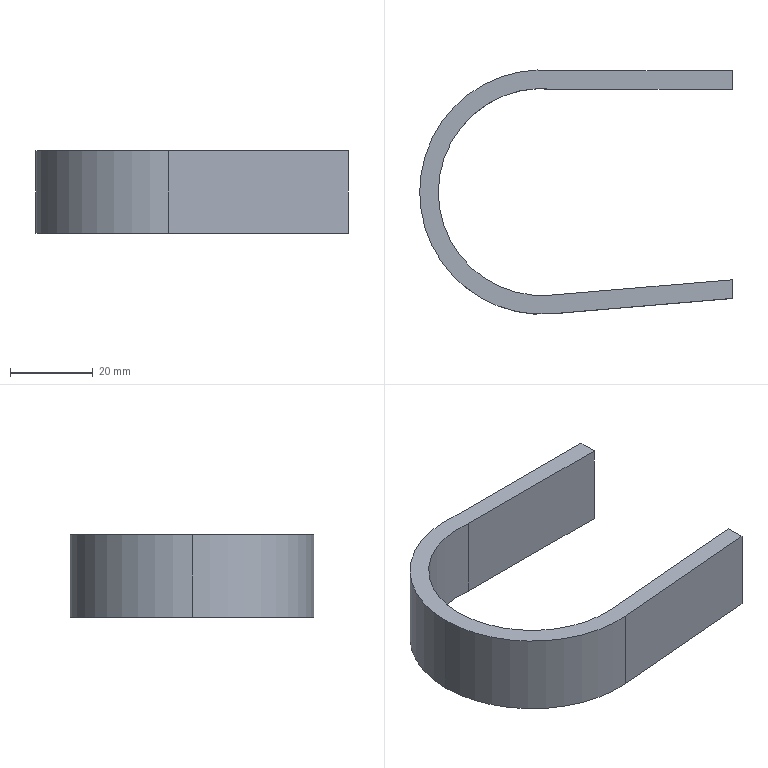Part | STEP file | Guide wheel mechanism revised.sldasm-Part-89 | 1 solid | 12 faces | box 75.5 x 59 x 20 mm | volume 15993 mm3 | plane 8 | cylinder 4 | commonest cylinder face diameters 50 x2 59 x2
STEP:
#1=CARTESIAN_POINT('',(-32.907,-0.3917,10.));
#2=VERTEX_POINT('',#1);
#3=CARTESIAN_POINT('',(-4.83,24.418,10.));
#4=VERTEX_POINT('',#3);
#5=CARTESIAN_POINT('',(-7.907,-0.3917,10.));
#6=DIRECTION('',(0.,0.,-1.));
#7=DIRECTION('',(1.,0.,0.));
#8=AXIS2_PLACEMENT_3D('',#5,#6,#7);
#9=CIRCLE('',#8,25.);
#10=EDGE_CURVE('',#2,#4,#9,.T.);
#11=ORIENTED_EDGE('',*,*,#10,.F.);
#12=CARTESIAN_POINT('',(-32.907,-0.3917,-10.));
#13=VERTEX_POINT('',#12);
#14=CARTESIAN_POINT('',(-32.907,-0.3917,10.));
#15=DIRECTION('',(0.,0.,-1.));
#16=VECTOR('',#15,1000.);
#17=LINE('',#14,#16);
#18=EDGE_CURVE('',#2,#13,#17,.T.);
#19=ORIENTED_EDGE('',*,*,#18,.T.);
#20=CARTESIAN_POINT('',(-4.83,24.418,-10.));
#21=VERTEX_POINT('',#20);
#22=CARTESIAN_POINT('',(-7.907,-0.3917,-10.));
#23=DIRECTION('',(0.,0.,-1.));
#24=DIRECTION('',(1.,0.,0.));
#25=AXIS2_PLACEMENT_3D('',#22,#23,#24);
#26=CIRCLE('',#25,25.);
#27=EDGE_CURVE('',#13,#21,#26,.T.);
#28=ORIENTED_EDGE('',*,*,#27,.T.);
#29=CARTESIAN_POINT('',(-4.83,24.418,10.));
#30=DIRECTION('',(0.,0.,-1.));
#31=VECTOR('',#30,1000.);
#32=LINE('',#29,#31);
#33=EDGE_CURVE('',#4,#21,#32,.T.);
#34=ORIENTED_EDGE('',*,*,#33,.F.);
#35=EDGE_LOOP('',(#11,#19,#28,#34));
#36=FACE_OUTER_BOUND('',#35,.T.);
#37=CARTESIAN_POINT('',(-7.907,-0.3917,10.));
#38=DIRECTION('',(0.,0.,-1.));
#39=DIRECTION('',(-1.,0.,0.));
#40=AXIS2_PLACEMENT_3D('',#37,#38,#39);
#41=CYLINDRICAL_SURFACE('',#40,25.);
#42=ADVANCED_FACE('',(#36),#41,.F.);
#43=CARTESIAN_POINT('',(-37.407,-0.3917,10.));
#44=VERTEX_POINT('',#43);
#45=CARTESIAN_POINT('',(-5.405,-29.785,10.));
#46=VERTEX_POINT('',#45);
#47=CARTESIAN_POINT('',(-7.907,-0.3917,10.));
#48=DIRECTION('',(0.,0.,1.));
#49=DIRECTION('',(1.,0.,0.));
#50=AXIS2_PLACEMENT_3D('',#47,#48,#49);
#51=CIRCLE('',#50,29.5);
#52=EDGE_CURVE('',#44,#46,#51,.T.);
#53=ORIENTED_EDGE('',*,*,#52,.F.);
#54=CARTESIAN_POINT('',(-37.407,-0.3917,-10.));
#55=VERTEX_POINT('',#54);
#56=CARTESIAN_POINT('',(-37.407,-0.3917,10.));
#57=DIRECTION('',(0.,0.,-1.));
#58=VECTOR('',#57,1000.);
#59=LINE('',#56,#58);
#60=EDGE_CURVE('',#44,#55,#59,.T.);
#61=ORIENTED_EDGE('',*,*,#60,.T.);
#62=CARTESIAN_POINT('',(-5.405,-29.785,-10.));
#63=VERTEX_POINT('',#62);
#64=CARTESIAN_POINT('',(-7.907,-0.3917,-10.));
#65=DIRECTION('',(0.,0.,1.));
#66=DIRECTION('',(1.,0.,0.));
#67=AXIS2_PLACEMENT_3D('',#64,#65,#66);
#68=CIRCLE('',#67,29.5);
#69=EDGE_CURVE('',#55,#63,#68,.T.);
#70=ORIENTED_EDGE('',*,*,#69,.T.);
#71=CARTESIAN_POINT('',(-5.405,-29.785,10.));
#72=DIRECTION('',(0.,0.,-1.));
#73=VECTOR('',#72,1000.);
#74=LINE('',#71,#73);
#75=EDGE_CURVE('',#46,#63,#74,.T.);
#76=ORIENTED_EDGE('',*,*,#75,.F.);
#77=EDGE_LOOP('',(#53,#61,#70,#76));
#78=FACE_OUTER_BOUND('',#77,.T.);
#79=CARTESIAN_POINT('',(-7.907,-0.3917,10.));
#80=DIRECTION('',(0.,0.,-1.));
#81=DIRECTION('',(-1.,0.,0.));
#82=AXIS2_PLACEMENT_3D('',#79,#80,#81);
#83=CYLINDRICAL_SURFACE('',#82,29.5);
#84=ADVANCED_FACE('',(#78),#83,.T.);
#85=CARTESIAN_POINT('',(38.093,24.418,-10.));
#86=VERTEX_POINT('',#85);
#87=CARTESIAN_POINT('',(38.093,28.918,-10.));
#88=VERTEX_POINT('',#87);
#89=CARTESIAN_POINT('',(38.093,28.918,-10.));
#90=DIRECTION('',(0.,1.,0.));
#91=VECTOR('',#90,1000.);
#92=LINE('',#89,#91);
#93=EDGE_CURVE('',#86,#88,#92,.T.);
#94=ORIENTED_EDGE('',*,*,#93,.T.);
#95=CARTESIAN_POINT('',(38.093,28.918,10.));
#96=VERTEX_POINT('',#95);
#97=CARTESIAN_POINT('',(38.093,28.918,10.));
#98=DIRECTION('',(0.,0.,-1.));
#99=VECTOR('',#98,1000.);
#100=LINE('',#97,#99);
#101=EDGE_CURVE('',#96,#88,#100,.T.);
#102=ORIENTED_EDGE('',*,*,#101,.F.);
#103=CARTESIAN_POINT('',(38.093,24.418,10.));
#104=VERTEX_POINT('',#103);
#105=CARTESIAN_POINT('',(38.093,28.918,10.));
#106=DIRECTION('',(0.,1.,0.));
#107=VECTOR('',#106,1000.);
#108=LINE('',#105,#107);
#109=EDGE_CURVE('',#104,#96,#108,.T.);
#110=ORIENTED_EDGE('',*,*,#109,.F.);
#111=CARTESIAN_POINT('',(38.093,24.418,10.));
#112=DIRECTION('',(0.,0.,-1.));
#113=VECTOR('',#112,1000.);
#114=LINE('',#111,#113);
#115=EDGE_CURVE('',#104,#86,#114,.T.);
#116=ORIENTED_EDGE('',*,*,#115,.T.);
#117=EDGE_LOOP('',(#94,#102,#110,#116));
#118=FACE_OUTER_BOUND('',#117,.T.);
#119=CARTESIAN_POINT('',(38.093,28.918,10.));
#120=DIRECTION('',(-1.,0.,0.));
#121=DIRECTION('',(0.,0.,1.));
#122=AXIS2_PLACEMENT_3D('',#119,#120,#121);
#123=PLANE('',#122);
#124=ADVANCED_FACE('',(#118),#123,.F.);
#125=CARTESIAN_POINT('',(-4.564,28.918,-10.));
#126=VERTEX_POINT('',#125);
#127=CARTESIAN_POINT('',(38.093,28.918,-10.));
#128=DIRECTION('',(-1.,0.,0.));
#129=VECTOR('',#128,1000.);
#130=LINE('',#127,#129);
#131=EDGE_CURVE('',#88,#126,#130,.T.);
#132=ORIENTED_EDGE('',*,*,#131,.T.);
#133=CARTESIAN_POINT('',(-4.564,28.918,10.));
#134=VERTEX_POINT('',#133);
#135=CARTESIAN_POINT('',(-4.564,28.918,10.));
#136=DIRECTION('',(0.,0.,-1.));
#137=VECTOR('',#136,1000.);
#138=LINE('',#135,#137);
#139=EDGE_CURVE('',#134,#126,#138,.T.);
#140=ORIENTED_EDGE('',*,*,#139,.F.);
#141=CARTESIAN_POINT('',(38.093,28.918,10.));
#142=DIRECTION('',(-1.,0.,0.));
#143=VECTOR('',#142,1000.);
#144=LINE('',#141,#143);
#145=EDGE_CURVE('',#96,#134,#144,.T.);
#146=ORIENTED_EDGE('',*,*,#145,.F.);
#147=ORIENTED_EDGE('',*,*,#101,.T.);
#148=EDGE_LOOP('',(#132,#140,#146,#147));
#149=FACE_OUTER_BOUND('',#148,.T.);
#150=CARTESIAN_POINT('',(38.093,28.918,10.));
#151=DIRECTION('',(0.,-1.,0.));
#152=DIRECTION('',(1.,0.,0.));
#153=AXIS2_PLACEMENT_3D('',#150,#151,#152);
#154=PLANE('',#153);
#155=ADVANCED_FACE('',(#149),#154,.F.);
#156=ORIENTED_EDGE('',*,*,#60,.F.);
#157=CARTESIAN_POINT('',(-7.907,-0.3917,10.));
#158=DIRECTION('',(0.,0.,1.));
#159=DIRECTION('',(1.,0.,0.));
#160=AXIS2_PLACEMENT_3D('',#157,#158,#159);
#161=CIRCLE('',#160,29.5);
#162=EDGE_CURVE('',#134,#44,#161,.T.);
#163=ORIENTED_EDGE('',*,*,#162,.F.);
#164=ORIENTED_EDGE('',*,*,#139,.T.);
#165=CARTESIAN_POINT('',(-7.907,-0.3917,-10.));
#166=DIRECTION('',(0.,0.,1.));
#167=DIRECTION('',(1.,0.,0.));
#168=AXIS2_PLACEMENT_3D('',#165,#166,#167);
#169=CIRCLE('',#168,29.5);
#170=EDGE_CURVE('',#126,#55,#169,.T.);
#171=ORIENTED_EDGE('',*,*,#170,.T.);
#172=EDGE_LOOP('',(#156,#163,#164,#171));
#173=FACE_OUTER_BOUND('',#172,.T.);
#174=CARTESIAN_POINT('',(-7.907,-0.3917,10.));
#175=DIRECTION('',(0.,0.,-1.));
#176=DIRECTION('',(-1.,0.,0.));
#177=AXIS2_PLACEMENT_3D('',#174,#175,#176);
#178=CYLINDRICAL_SURFACE('',#177,29.5);
#179=ADVANCED_FACE('',(#173),#178,.T.);
#180=CARTESIAN_POINT('',(38.093,-26.082,-10.));
#181=VERTEX_POINT('',#180);
#182=CARTESIAN_POINT('',(38.093,-26.082,-10.));
#183=DIRECTION('',(0.9964,0.08484,0.));
#184=VECTOR('',#183,1000.);
#185=LINE('',#182,#184);
#186=EDGE_CURVE('',#63,#181,#185,.T.);
#187=ORIENTED_EDGE('',*,*,#186,.T.);
#188=CARTESIAN_POINT('',(38.093,-26.082,10.));
#189=VERTEX_POINT('',#188);
#190=CARTESIAN_POINT('',(38.093,-26.082,10.));
#191=DIRECTION('',(0.,0.,-1.));
#192=VECTOR('',#191,1000.);
#193=LINE('',#190,#192);
#194=EDGE_CURVE('',#189,#181,#193,.T.);
#195=ORIENTED_EDGE('',*,*,#194,.F.);
#196=CARTESIAN_POINT('',(38.093,-26.082,10.));
#197=DIRECTION('',(0.9964,0.08484,0.));
#198=VECTOR('',#197,1000.);
#199=LINE('',#196,#198);
#200=EDGE_CURVE('',#46,#189,#199,.T.);
#201=ORIENTED_EDGE('',*,*,#200,.F.);
#202=ORIENTED_EDGE('',*,*,#75,.T.);
#203=EDGE_LOOP('',(#187,#195,#201,#202));
#204=FACE_OUTER_BOUND('',#203,.T.);
#205=CARTESIAN_POINT('',(38.093,-26.082,10.));
#206=DIRECTION('',(-0.08484,0.9964,0.));
#207=DIRECTION('',(-0.9964,-0.08484,0.));
#208=AXIS2_PLACEMENT_3D('',#205,#206,#207);
#209=PLANE('',#208);
#210=ADVANCED_FACE('',(#204),#209,.F.);
#211=CARTESIAN_POINT('',(38.093,-21.582,-10.));
#212=VERTEX_POINT('',#211);
#213=CARTESIAN_POINT('',(38.093,-21.582,-10.));
#214=DIRECTION('',(0.,1.,0.));
#215=VECTOR('',#214,1000.);
#216=LINE('',#213,#215);
#217=EDGE_CURVE('',#181,#212,#216,.T.);
#218=ORIENTED_EDGE('',*,*,#217,.T.);
#219=CARTESIAN_POINT('',(38.093,-21.582,10.));
#220=VERTEX_POINT('',#219);
#221=CARTESIAN_POINT('',(38.093,-21.582,10.));
#222=DIRECTION('',(0.,0.,-1.));
#223=VECTOR('',#222,1000.);
#224=LINE('',#221,#223);
#225=EDGE_CURVE('',#220,#212,#224,.T.);
#226=ORIENTED_EDGE('',*,*,#225,.F.);
#227=CARTESIAN_POINT('',(38.093,-21.582,10.));
#228=DIRECTION('',(0.,1.,0.));
#229=VECTOR('',#228,1000.);
#230=LINE('',#227,#229);
#231=EDGE_CURVE('',#189,#220,#230,.T.);
#232=ORIENTED_EDGE('',*,*,#231,.F.);
#233=ORIENTED_EDGE('',*,*,#194,.T.);
#234=EDGE_LOOP('',(#218,#226,#232,#233));
#235=FACE_OUTER_BOUND('',#234,.T.);
#236=CARTESIAN_POINT('',(38.093,-21.582,10.));
#237=DIRECTION('',(-1.,0.,0.));
#238=DIRECTION('',(0.,0.,1.));
#239=AXIS2_PLACEMENT_3D('',#236,#237,#238);
#240=PLANE('',#239);
#241=ADVANCED_FACE('',(#235),#240,.F.);
#242=CARTESIAN_POINT('',(-5.796,-25.302,-10.));
#243=VERTEX_POINT('',#242);
#244=CARTESIAN_POINT('',(38.093,-21.582,-10.));
#245=DIRECTION('',(-0.9964,-0.08447,0.));
#246=VECTOR('',#245,1000.);
#247=LINE('',#244,#246);
#248=EDGE_CURVE('',#212,#243,#247,.T.);
#249=ORIENTED_EDGE('',*,*,#248,.T.);
#250=CARTESIAN_POINT('',(-5.796,-25.302,10.));
#251=VERTEX_POINT('',#250);
#252=CARTESIAN_POINT('',(-5.796,-25.302,10.));
#253=DIRECTION('',(0.,0.,-1.));
#254=VECTOR('',#253,1000.);
#255=LINE('',#252,#254);
#256=EDGE_CURVE('',#251,#243,#255,.T.);
#257=ORIENTED_EDGE('',*,*,#256,.F.);
#258=CARTESIAN_POINT('',(38.093,-21.582,10.));
#259=DIRECTION('',(-0.9964,-0.08447,0.));
#260=VECTOR('',#259,1000.);
#261=LINE('',#258,#260);
#262=EDGE_CURVE('',#220,#251,#261,.T.);
#263=ORIENTED_EDGE('',*,*,#262,.F.);
#264=ORIENTED_EDGE('',*,*,#225,.T.);
#265=EDGE_LOOP('',(#249,#257,#263,#264));
#266=FACE_OUTER_BOUND('',#265,.T.);
#267=CARTESIAN_POINT('',(38.093,-21.582,10.));
#268=DIRECTION('',(0.08447,-0.9964,0.));
#269=DIRECTION('',(0.9964,0.08447,0.));
#270=AXIS2_PLACEMENT_3D('',#267,#268,#269);
#271=PLANE('',#270);
#272=ADVANCED_FACE('',(#266),#271,.F.);
#273=ORIENTED_EDGE('',*,*,#18,.F.);
#274=CARTESIAN_POINT('',(-7.907,-0.3917,10.));
#275=DIRECTION('',(0.,0.,-1.));
#276=DIRECTION('',(1.,0.,0.));
#277=AXIS2_PLACEMENT_3D('',#274,#275,#276);
#278=CIRCLE('',#277,25.);
#279=EDGE_CURVE('',#251,#2,#278,.T.);
#280=ORIENTED_EDGE('',*,*,#279,.F.);
#281=ORIENTED_EDGE('',*,*,#256,.T.);
#282=CARTESIAN_POINT('',(-7.907,-0.3917,-10.));
#283=DIRECTION('',(0.,0.,-1.));
#284=DIRECTION('',(1.,0.,0.));
#285=AXIS2_PLACEMENT_3D('',#282,#283,#284);
#286=CIRCLE('',#285,25.);
#287=EDGE_CURVE('',#243,#13,#286,.T.);
#288=ORIENTED_EDGE('',*,*,#287,.T.);
#289=EDGE_LOOP('',(#273,#280,#281,#288));
#290=FACE_OUTER_BOUND('',#289,.T.);
#291=CARTESIAN_POINT('',(-7.907,-0.3917,10.));
#292=DIRECTION('',(0.,0.,-1.));
#293=DIRECTION('',(-1.,0.,0.));
#294=AXIS2_PLACEMENT_3D('',#291,#292,#293);
#295=CYLINDRICAL_SURFACE('',#294,25.);
#296=ADVANCED_FACE('',(#290),#295,.F.);
#297=CARTESIAN_POINT('',(38.093,24.418,-10.));
#298=DIRECTION('',(1.,0.,0.));
#299=VECTOR('',#298,1000.);
#300=LINE('',#297,#299);
#301=EDGE_CURVE('',#21,#86,#300,.T.);
#302=ORIENTED_EDGE('',*,*,#301,.T.);
#303=ORIENTED_EDGE('',*,*,#115,.F.);
#304=CARTESIAN_POINT('',(38.093,24.418,10.));
#305=DIRECTION('',(1.,0.,0.));
#306=VECTOR('',#305,1000.);
#307=LINE('',#304,#306);
#308=EDGE_CURVE('',#4,#104,#307,.T.);
#309=ORIENTED_EDGE('',*,*,#308,.F.);
#310=ORIENTED_EDGE('',*,*,#33,.T.);
#311=EDGE_LOOP('',(#302,#303,#309,#310));
#312=FACE_OUTER_BOUND('',#311,.T.);
#313=CARTESIAN_POINT('',(38.093,24.418,10.));
#314=DIRECTION('',(0.,1.,0.));
#315=DIRECTION('',(-1.,0.,0.));
#316=AXIS2_PLACEMENT_3D('',#313,#314,#315);
#317=PLANE('',#316);
#318=ADVANCED_FACE('',(#312),#317,.F.);
#319=ORIENTED_EDGE('',*,*,#109,.T.);
#320=ORIENTED_EDGE('',*,*,#145,.T.);
#321=ORIENTED_EDGE('',*,*,#162,.T.);
#322=ORIENTED_EDGE('',*,*,#52,.T.);
#323=ORIENTED_EDGE('',*,*,#200,.T.);
#324=ORIENTED_EDGE('',*,*,#231,.T.);
#325=ORIENTED_EDGE('',*,*,#262,.T.);
#326=ORIENTED_EDGE('',*,*,#279,.T.);
#327=ORIENTED_EDGE('',*,*,#10,.T.);
#328=ORIENTED_EDGE('',*,*,#308,.T.);
#329=EDGE_LOOP('',(#319,#320,#321,#322,#323,#324,#325,#326,#327,#328));
#330=FACE_OUTER_BOUND('',#329,.T.);
#331=CARTESIAN_POINT('',(-7.907,-0.3917,10.));
#332=DIRECTION('',(0.,0.,1.));
#333=DIRECTION('',(1.,0.,0.));
#334=AXIS2_PLACEMENT_3D('',#331,#332,#333);
#335=PLANE('',#334);
#336=ADVANCED_FACE('',(#330),#335,.T.);
#337=ORIENTED_EDGE('',*,*,#93,.F.);
#338=ORIENTED_EDGE('',*,*,#301,.F.);
#339=ORIENTED_EDGE('',*,*,#27,.F.);
#340=ORIENTED_EDGE('',*,*,#287,.F.);
#341=ORIENTED_EDGE('',*,*,#248,.F.);
#342=ORIENTED_EDGE('',*,*,#217,.F.);
#343=ORIENTED_EDGE('',*,*,#186,.F.);
#344=ORIENTED_EDGE('',*,*,#69,.F.);
#345=ORIENTED_EDGE('',*,*,#170,.F.);
#346=ORIENTED_EDGE('',*,*,#131,.F.);
#347=EDGE_LOOP('',(#337,#338,#339,#340,#341,#342,#343,#344,#345,#346));
#348=FACE_OUTER_BOUND('',#347,.T.);
#349=CARTESIAN_POINT('',(-7.907,-0.3917,-10.));
#350=DIRECTION('',(0.,0.,1.));
#351=DIRECTION('',(1.,0.,0.));
#352=AXIS2_PLACEMENT_3D('',#349,#350,#351);
#353=PLANE('',#352);
#354=ADVANCED_FACE('',(#348),#353,.F.);
#355=CLOSED_SHELL('',(#42,#84,#124,#155,#179,#210,#241,#272,#296,#318,#336,#354));
#356=MANIFOLD_SOLID_BREP('',#355);
#357=CARTESIAN_POINT('',(0.,0.,0.));
#358=DIRECTION('',(0.,0.,1.));
#359=DIRECTION('',(1.,0.,0.));
#360=AXIS2_PLACEMENT_3D('',#357,#358,#359);
#361=(LENGTH_UNIT()NAMED_UNIT(*)SI_UNIT(.MILLI.,.METRE.));
#362=UNCERTAINTY_MEASURE_WITH_UNIT(LENGTH_MEASURE(0.00001),#361,'','');
#363=(NAMED_UNIT(*)PLANE_ANGLE_UNIT()SI_UNIT($,.RADIAN.));
#364=(NAMED_UNIT(*)SI_UNIT($,.STERADIAN.)SOLID_ANGLE_UNIT());
#365=(GEOMETRIC_REPRESENTATION_CONTEXT(3)GLOBAL_UNCERTAINTY_ASSIGNED_CONTEXT((#362))GLOBAL_UNIT_ASSIGNED_CONTEXT((#361,#363,#364))REPRESENTATION_CONTEXT('',''));
#366=ADVANCED_BREP_SHAPE_REPRESENTATION('',(#356,#360),#365);